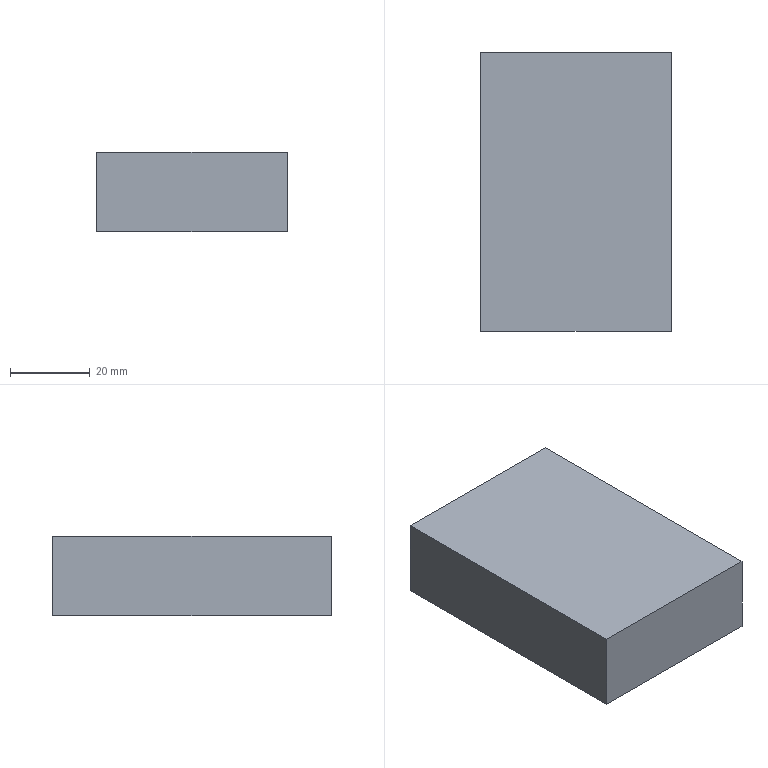Part | STEP file | Spacer block 4 | 1 solid | 6 faces | box 48 x 70 x 20 mm | volume 67200 mm3 | plane 6
STEP:
#1=CARTESIAN_POINT('',(-90.745,-35.,0.));
#2=VERTEX_POINT('',#1);
#3=CARTESIAN_POINT('',(-42.745,-35.,0.));
#4=VERTEX_POINT('',#3);
#5=CARTESIAN_POINT('',(-90.745,-35.,0.));
#6=DIRECTION('',(1.,0.,0.));
#7=VECTOR('',#6,1000.);
#8=LINE('',#5,#7);
#9=EDGE_CURVE('',#2,#4,#8,.T.);
#10=ORIENTED_EDGE('',*,*,#9,.T.);
#11=CARTESIAN_POINT('',(-42.745,-35.,20.));
#12=VERTEX_POINT('',#11);
#13=CARTESIAN_POINT('',(-42.745,-35.,20.));
#14=DIRECTION('',(0.,0.,-1.));
#15=VECTOR('',#14,1000.);
#16=LINE('',#13,#15);
#17=EDGE_CURVE('',#12,#4,#16,.T.);
#18=ORIENTED_EDGE('',*,*,#17,.F.);
#19=CARTESIAN_POINT('',(-90.745,-35.,20.));
#20=VERTEX_POINT('',#19);
#21=CARTESIAN_POINT('',(-90.745,-35.,20.));
#22=DIRECTION('',(1.,0.,0.));
#23=VECTOR('',#22,1000.);
#24=LINE('',#21,#23);
#25=EDGE_CURVE('',#20,#12,#24,.T.);
#26=ORIENTED_EDGE('',*,*,#25,.F.);
#27=CARTESIAN_POINT('',(-90.745,-35.,20.));
#28=DIRECTION('',(0.,0.,-1.));
#29=VECTOR('',#28,1000.);
#30=LINE('',#27,#29);
#31=EDGE_CURVE('',#20,#2,#30,.T.);
#32=ORIENTED_EDGE('',*,*,#31,.T.);
#33=EDGE_LOOP('',(#10,#18,#26,#32));
#34=FACE_OUTER_BOUND('',#33,.T.);
#35=CARTESIAN_POINT('',(-90.745,-35.,20.));
#36=DIRECTION('',(0.,1.,0.));
#37=DIRECTION('',(0.,0.,1.));
#38=AXIS2_PLACEMENT_3D('',#35,#36,#37);
#39=PLANE('',#38);
#40=ADVANCED_FACE('',(#34),#39,.F.);
#41=CARTESIAN_POINT('',(-42.745,35.,0.));
#42=VERTEX_POINT('',#41);
#43=CARTESIAN_POINT('',(-42.745,-35.,0.));
#44=DIRECTION('',(0.,1.,0.));
#45=VECTOR('',#44,1000.);
#46=LINE('',#43,#45);
#47=EDGE_CURVE('',#4,#42,#46,.T.);
#48=ORIENTED_EDGE('',*,*,#47,.T.);
#49=CARTESIAN_POINT('',(-42.745,35.,20.));
#50=VERTEX_POINT('',#49);
#51=CARTESIAN_POINT('',(-42.745,35.,20.));
#52=DIRECTION('',(0.,0.,-1.));
#53=VECTOR('',#52,1000.);
#54=LINE('',#51,#53);
#55=EDGE_CURVE('',#50,#42,#54,.T.);
#56=ORIENTED_EDGE('',*,*,#55,.F.);
#57=CARTESIAN_POINT('',(-42.745,-35.,20.));
#58=DIRECTION('',(0.,1.,0.));
#59=VECTOR('',#58,1000.);
#60=LINE('',#57,#59);
#61=EDGE_CURVE('',#12,#50,#60,.T.);
#62=ORIENTED_EDGE('',*,*,#61,.F.);
#63=ORIENTED_EDGE('',*,*,#17,.T.);
#64=EDGE_LOOP('',(#48,#56,#62,#63));
#65=FACE_OUTER_BOUND('',#64,.T.);
#66=CARTESIAN_POINT('',(-42.745,-35.,20.));
#67=DIRECTION('',(-1.,0.,0.));
#68=DIRECTION('',(0.,-1.,0.));
#69=AXIS2_PLACEMENT_3D('',#66,#67,#68);
#70=PLANE('',#69);
#71=ADVANCED_FACE('',(#65),#70,.F.);
#72=CARTESIAN_POINT('',(-90.745,35.,0.));
#73=VERTEX_POINT('',#72);
#74=CARTESIAN_POINT('',(-90.745,35.,0.));
#75=DIRECTION('',(1.,0.,0.));
#76=VECTOR('',#75,1000.);
#77=LINE('',#74,#76);
#78=EDGE_CURVE('',#73,#42,#77,.T.);
#79=ORIENTED_EDGE('',*,*,#78,.F.);
#80=CARTESIAN_POINT('',(-90.745,35.,20.));
#81=VERTEX_POINT('',#80);
#82=CARTESIAN_POINT('',(-90.745,35.,20.));
#83=DIRECTION('',(0.,0.,-1.));
#84=VECTOR('',#83,1000.);
#85=LINE('',#82,#84);
#86=EDGE_CURVE('',#81,#73,#85,.T.);
#87=ORIENTED_EDGE('',*,*,#86,.F.);
#88=CARTESIAN_POINT('',(-90.745,35.,20.));
#89=DIRECTION('',(1.,0.,0.));
#90=VECTOR('',#89,1000.);
#91=LINE('',#88,#90);
#92=EDGE_CURVE('',#81,#50,#91,.T.);
#93=ORIENTED_EDGE('',*,*,#92,.T.);
#94=ORIENTED_EDGE('',*,*,#55,.T.);
#95=EDGE_LOOP('',(#79,#87,#93,#94));
#96=FACE_OUTER_BOUND('',#95,.T.);
#97=CARTESIAN_POINT('',(-90.745,35.,20.));
#98=DIRECTION('',(0.,1.,0.));
#99=DIRECTION('',(-1.,0.,0.));
#100=AXIS2_PLACEMENT_3D('',#97,#98,#99);
#101=PLANE('',#100);
#102=ADVANCED_FACE('',(#96),#101,.T.);
#103=CARTESIAN_POINT('',(-90.745,-35.,0.));
#104=DIRECTION('',(0.,1.,0.));
#105=VECTOR('',#104,1000.);
#106=LINE('',#103,#105);
#107=EDGE_CURVE('',#2,#73,#106,.T.);
#108=ORIENTED_EDGE('',*,*,#107,.F.);
#109=ORIENTED_EDGE('',*,*,#31,.F.);
#110=CARTESIAN_POINT('',(-90.745,-35.,20.));
#111=DIRECTION('',(0.,1.,0.));
#112=VECTOR('',#111,1000.);
#113=LINE('',#110,#112);
#114=EDGE_CURVE('',#20,#81,#113,.T.);
#115=ORIENTED_EDGE('',*,*,#114,.T.);
#116=ORIENTED_EDGE('',*,*,#86,.T.);
#117=EDGE_LOOP('',(#108,#109,#115,#116));
#118=FACE_OUTER_BOUND('',#117,.T.);
#119=CARTESIAN_POINT('',(-90.745,-35.,20.));
#120=DIRECTION('',(-1.,0.,0.));
#121=DIRECTION('',(0.,0.,1.));
#122=AXIS2_PLACEMENT_3D('',#119,#120,#121);
#123=PLANE('',#122);
#124=ADVANCED_FACE('',(#118),#123,.T.);
#125=ORIENTED_EDGE('',*,*,#25,.T.);
#126=ORIENTED_EDGE('',*,*,#61,.T.);
#127=ORIENTED_EDGE('',*,*,#92,.F.);
#128=ORIENTED_EDGE('',*,*,#114,.F.);
#129=EDGE_LOOP('',(#125,#126,#127,#128));
#130=FACE_OUTER_BOUND('',#129,.T.);
#131=CARTESIAN_POINT('',(0.,0.,20.));
#132=DIRECTION('',(0.,0.,1.));
#133=DIRECTION('',(1.,0.,0.));
#134=AXIS2_PLACEMENT_3D('',#131,#132,#133);
#135=PLANE('',#134);
#136=ADVANCED_FACE('',(#130),#135,.T.);
#137=ORIENTED_EDGE('',*,*,#9,.F.);
#138=ORIENTED_EDGE('',*,*,#107,.T.);
#139=ORIENTED_EDGE('',*,*,#78,.T.);
#140=ORIENTED_EDGE('',*,*,#47,.F.);
#141=EDGE_LOOP('',(#137,#138,#139,#140));
#142=FACE_OUTER_BOUND('',#141,.T.);
#143=CARTESIAN_POINT('',(0.,0.,0.));
#144=DIRECTION('',(0.,0.,1.));
#145=DIRECTION('',(1.,0.,0.));
#146=AXIS2_PLACEMENT_3D('',#143,#144,#145);
#147=PLANE('',#146);
#148=ADVANCED_FACE('',(#142),#147,.F.);
#149=CLOSED_SHELL('',(#40,#71,#102,#124,#136,#148));
#150=MANIFOLD_SOLID_BREP('',#149);
#151=CARTESIAN_POINT('',(0.,0.,0.));
#152=DIRECTION('',(0.,0.,1.));
#153=DIRECTION('',(1.,0.,0.));
#154=AXIS2_PLACEMENT_3D('',#151,#152,#153);
#155=(LENGTH_UNIT()NAMED_UNIT(*)SI_UNIT(.MILLI.,.METRE.));
#156=UNCERTAINTY_MEASURE_WITH_UNIT(LENGTH_MEASURE(0.00001),#155,'','');
#157=(NAMED_UNIT(*)PLANE_ANGLE_UNIT()SI_UNIT($,.RADIAN.));
#158=(NAMED_UNIT(*)SI_UNIT($,.STERADIAN.)SOLID_ANGLE_UNIT());
#159=(GEOMETRIC_REPRESENTATION_CONTEXT(3)GLOBAL_UNCERTAINTY_ASSIGNED_CONTEXT((#156))GLOBAL_UNIT_ASSIGNED_CONTEXT((#155,#157,#158))REPRESENTATION_CONTEXT('',''));
#160=ADVANCED_BREP_SHAPE_REPRESENTATION('',(#150,#154),#159);